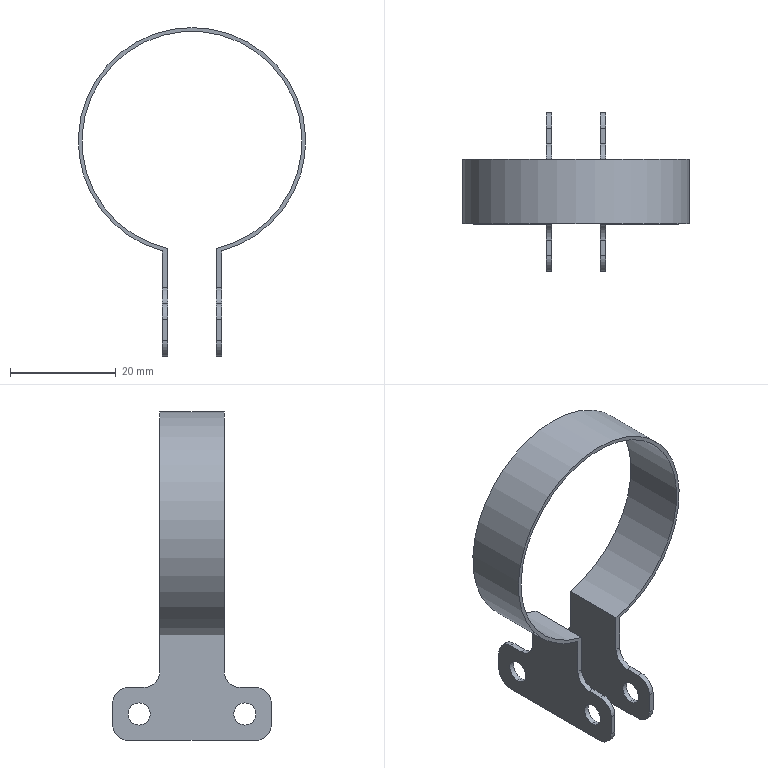Part | SolidWorks | features Extrusion 1, ICE 1, MirrorPattern 1 | 1 solid | 38 faces | box 43 x 30 x 62.202 mm | volume 1832 mm3 | cylinder 22 | plane 16 | commonest cylinder face diameters 6 x12 4.2 x8 41.6 x1 43 x1
STEP:
#1=CARTESIAN_POINT('',(5.6,16.1,-33.602));
#2=VERTEX_POINT('',#1);
#3=CARTESIAN_POINT('',(5.6,16.1,-37.802));
#4=VERTEX_POINT('',#3);
#5=CARTESIAN_POINT('',(5.6,16.1,-35.702));
#6=DIRECTION('',(1.,0.,0.));
#7=DIRECTION('',(0.,0.,-1.));
#8=AXIS2_PLACEMENT_3D('',#5,#6,#7);
#9=CIRCLE('',#8,2.1);
#10=EDGE_CURVE('',#2,#4,#9,.T.);
#11=ORIENTED_EDGE('',*,*,#10,.T.);
#12=CARTESIAN_POINT('',(4.6,16.1,-37.802));
#13=VERTEX_POINT('',#12);
#14=CARTESIAN_POINT('',(5.6,16.1,-37.802));
#15=DIRECTION('',(-1.,0.,0.));
#16=VECTOR('',#15,1000.);
#17=LINE('',#14,#16);
#18=EDGE_CURVE('',#4,#13,#17,.T.);
#19=ORIENTED_EDGE('',*,*,#18,.T.);
#20=CARTESIAN_POINT('',(4.6,16.1,-33.602));
#21=VERTEX_POINT('',#20);
#22=CARTESIAN_POINT('',(4.6,16.1,-35.702));
#23=DIRECTION('',(1.,0.,0.));
#24=DIRECTION('',(0.,0.,-1.));
#25=AXIS2_PLACEMENT_3D('',#22,#23,#24);
#26=CIRCLE('',#25,2.1);
#27=EDGE_CURVE('',#21,#13,#26,.T.);
#28=ORIENTED_EDGE('',*,*,#27,.F.);
#29=CARTESIAN_POINT('',(5.6,16.1,-33.602));
#30=DIRECTION('',(-1.,0.,0.));
#31=VECTOR('',#30,1000.);
#32=LINE('',#29,#31);
#33=EDGE_CURVE('',#2,#21,#32,.T.);
#34=ORIENTED_EDGE('',*,*,#33,.F.);
#35=EDGE_LOOP('',(#11,#19,#28,#34));
#36=FACE_OUTER_BOUND('',#35,.T.);
#37=CARTESIAN_POINT('',(5.6,16.1,-35.702));
#38=DIRECTION('',(-1.,0.,0.));
#39=DIRECTION('',(0.,0.,1.));
#40=AXIS2_PLACEMENT_3D('',#37,#38,#39);
#41=CYLINDRICAL_SURFACE('',#40,2.1);
#42=ADVANCED_FACE('',(#36),#41,.F.);
#43=CARTESIAN_POINT('',(5.6,-3.9,-33.602));
#44=VERTEX_POINT('',#43);
#45=CARTESIAN_POINT('',(5.6,-3.9,-37.802));
#46=VERTEX_POINT('',#45);
#47=CARTESIAN_POINT('',(5.6,-3.9,-35.702));
#48=DIRECTION('',(1.,0.,0.));
#49=DIRECTION('',(0.,0.,-1.));
#50=AXIS2_PLACEMENT_3D('',#47,#48,#49);
#51=CIRCLE('',#50,2.1);
#52=EDGE_CURVE('',#44,#46,#51,.T.);
#53=ORIENTED_EDGE('',*,*,#52,.T.);
#54=CARTESIAN_POINT('',(4.6,-3.9,-37.802));
#55=VERTEX_POINT('',#54);
#56=CARTESIAN_POINT('',(5.6,-3.9,-37.802));
#57=DIRECTION('',(-1.,0.,0.));
#58=VECTOR('',#57,1000.);
#59=LINE('',#56,#58);
#60=EDGE_CURVE('',#46,#55,#59,.T.);
#61=ORIENTED_EDGE('',*,*,#60,.T.);
#62=CARTESIAN_POINT('',(4.6,-3.9,-33.602));
#63=VERTEX_POINT('',#62);
#64=CARTESIAN_POINT('',(4.6,-3.9,-35.702));
#65=DIRECTION('',(1.,0.,0.));
#66=DIRECTION('',(0.,0.,-1.));
#67=AXIS2_PLACEMENT_3D('',#64,#65,#66);
#68=CIRCLE('',#67,2.1);
#69=EDGE_CURVE('',#63,#55,#68,.T.);
#70=ORIENTED_EDGE('',*,*,#69,.F.);
#71=CARTESIAN_POINT('',(5.6,-3.9,-33.602));
#72=DIRECTION('',(-1.,0.,0.));
#73=VECTOR('',#72,1000.);
#74=LINE('',#71,#73);
#75=EDGE_CURVE('',#44,#63,#74,.T.);
#76=ORIENTED_EDGE('',*,*,#75,.F.);
#77=EDGE_LOOP('',(#53,#61,#70,#76));
#78=FACE_OUTER_BOUND('',#77,.T.);
#79=CARTESIAN_POINT('',(5.6,-3.9,-35.702));
#80=DIRECTION('',(-1.,0.,0.));
#81=DIRECTION('',(0.,0.,1.));
#82=AXIS2_PLACEMENT_3D('',#79,#80,#81);
#83=CYLINDRICAL_SURFACE('',#82,2.1);
#84=ADVANCED_FACE('',(#78),#83,.F.);
#85=CARTESIAN_POINT('',(-5.6,16.1,-33.602));
#86=VERTEX_POINT('',#85);
#87=CARTESIAN_POINT('',(-5.6,16.1,-37.802));
#88=VERTEX_POINT('',#87);
#89=CARTESIAN_POINT('',(-5.6,16.1,-35.702));
#90=DIRECTION('',(1.,0.,0.));
#91=DIRECTION('',(0.,0.,-1.));
#92=AXIS2_PLACEMENT_3D('',#89,#90,#91);
#93=CIRCLE('',#92,2.1);
#94=EDGE_CURVE('',#86,#88,#93,.T.);
#95=ORIENTED_EDGE('',*,*,#94,.F.);
#96=CARTESIAN_POINT('',(-4.6,16.1,-33.602));
#97=VERTEX_POINT('',#96);
#98=CARTESIAN_POINT('',(-5.6,16.1,-33.602));
#99=DIRECTION('',(1.,0.,0.));
#100=VECTOR('',#99,1000.);
#101=LINE('',#98,#100);
#102=EDGE_CURVE('',#86,#97,#101,.T.);
#103=ORIENTED_EDGE('',*,*,#102,.T.);
#104=CARTESIAN_POINT('',(-4.6,16.1,-37.802));
#105=VERTEX_POINT('',#104);
#106=CARTESIAN_POINT('',(-4.6,16.1,-35.702));
#107=DIRECTION('',(1.,0.,0.));
#108=DIRECTION('',(0.,0.,-1.));
#109=AXIS2_PLACEMENT_3D('',#106,#107,#108);
#110=CIRCLE('',#109,2.1);
#111=EDGE_CURVE('',#97,#105,#110,.T.);
#112=ORIENTED_EDGE('',*,*,#111,.T.);
#113=CARTESIAN_POINT('',(-5.6,16.1,-37.802));
#114=DIRECTION('',(1.,0.,0.));
#115=VECTOR('',#114,1000.);
#116=LINE('',#113,#115);
#117=EDGE_CURVE('',#88,#105,#116,.T.);
#118=ORIENTED_EDGE('',*,*,#117,.F.);
#119=EDGE_LOOP('',(#95,#103,#112,#118));
#120=FACE_OUTER_BOUND('',#119,.T.);
#121=CARTESIAN_POINT('',(-5.6,16.1,-35.702));
#122=DIRECTION('',(1.,0.,0.));
#123=DIRECTION('',(0.,0.,-1.));
#124=AXIS2_PLACEMENT_3D('',#121,#122,#123);
#125=CYLINDRICAL_SURFACE('',#124,2.1);
#126=ADVANCED_FACE('',(#120),#125,.F.);
#127=CARTESIAN_POINT('',(-5.6,-3.9,-33.602));
#128=VERTEX_POINT('',#127);
#129=CARTESIAN_POINT('',(-5.6,-3.9,-37.802));
#130=VERTEX_POINT('',#129);
#131=CARTESIAN_POINT('',(-5.6,-3.9,-35.702));
#132=DIRECTION('',(1.,0.,0.));
#133=DIRECTION('',(0.,0.,-1.));
#134=AXIS2_PLACEMENT_3D('',#131,#132,#133);
#135=CIRCLE('',#134,2.1);
#136=EDGE_CURVE('',#128,#130,#135,.T.);
#137=ORIENTED_EDGE('',*,*,#136,.F.);
#138=CARTESIAN_POINT('',(-4.6,-3.9,-33.602));
#139=VERTEX_POINT('',#138);
#140=CARTESIAN_POINT('',(-5.6,-3.9,-33.602));
#141=DIRECTION('',(1.,0.,0.));
#142=VECTOR('',#141,1000.);
#143=LINE('',#140,#142);
#144=EDGE_CURVE('',#128,#139,#143,.T.);
#145=ORIENTED_EDGE('',*,*,#144,.T.);
#146=CARTESIAN_POINT('',(-4.6,-3.9,-37.802));
#147=VERTEX_POINT('',#146);
#148=CARTESIAN_POINT('',(-4.6,-3.9,-35.702));
#149=DIRECTION('',(1.,0.,0.));
#150=DIRECTION('',(0.,0.,-1.));
#151=AXIS2_PLACEMENT_3D('',#148,#149,#150);
#152=CIRCLE('',#151,2.1);
#153=EDGE_CURVE('',#139,#147,#152,.T.);
#154=ORIENTED_EDGE('',*,*,#153,.T.);
#155=CARTESIAN_POINT('',(-5.6,-3.9,-37.802));
#156=DIRECTION('',(1.,0.,0.));
#157=VECTOR('',#156,1000.);
#158=LINE('',#155,#157);
#159=EDGE_CURVE('',#130,#147,#158,.T.);
#160=ORIENTED_EDGE('',*,*,#159,.F.);
#161=EDGE_LOOP('',(#137,#145,#154,#160));
#162=FACE_OUTER_BOUND('',#161,.T.);
#163=CARTESIAN_POINT('',(-5.6,-3.9,-35.702));
#164=DIRECTION('',(1.,0.,0.));
#165=DIRECTION('',(0.,0.,-1.));
#166=AXIS2_PLACEMENT_3D('',#163,#164,#165);
#167=CYLINDRICAL_SURFACE('',#166,2.1);
#168=ADVANCED_FACE('',(#162),#167,.F.);
#169=CARTESIAN_POINT('',(5.6,12.2,-20.758));
#170=VERTEX_POINT('',#169);
#171=CARTESIAN_POINT('',(5.6,0.,-20.758));
#172=VERTEX_POINT('',#171);
#173=CARTESIAN_POINT('',(5.6,12.2,-20.758));
#174=DIRECTION('',(0.,-1.,0.));
#175=VECTOR('',#174,1000.);
#176=LINE('',#173,#175);
#177=EDGE_CURVE('',#170,#172,#176,.T.);
#178=ORIENTED_EDGE('',*,*,#177,.F.);
#179=CARTESIAN_POINT('',(-5.6,12.2,-20.758));
#180=VERTEX_POINT('',#179);
#181=CARTESIAN_POINT('',(0.,12.2,0.));
#182=DIRECTION('',(0.,1.,0.));
#183=DIRECTION('',(0.,0.,1.));
#184=AXIS2_PLACEMENT_3D('',#181,#182,#183);
#185=CIRCLE('',#184,21.5);
#186=EDGE_CURVE('',#180,#170,#185,.T.);
#187=ORIENTED_EDGE('',*,*,#186,.F.);
#188=CARTESIAN_POINT('',(-5.6,0.,-20.758));
#189=VERTEX_POINT('',#188);
#190=CARTESIAN_POINT('',(-5.6,12.2,-20.758));
#191=DIRECTION('',(0.,1.,0.));
#192=VECTOR('',#191,1000.);
#193=LINE('',#190,#192);
#194=EDGE_CURVE('',#189,#180,#193,.T.);
#195=ORIENTED_EDGE('',*,*,#194,.F.);
#196=CARTESIAN_POINT('',(0.,0.,0.));
#197=DIRECTION('',(0.,1.,0.));
#198=DIRECTION('',(0.,0.,1.));
#199=AXIS2_PLACEMENT_3D('',#196,#197,#198);
#200=CIRCLE('',#199,21.5);
#201=EDGE_CURVE('',#189,#172,#200,.T.);
#202=ORIENTED_EDGE('',*,*,#201,.T.);
#203=EDGE_LOOP('',(#178,#187,#195,#202));
#204=FACE_OUTER_BOUND('',#203,.T.);
#205=CARTESIAN_POINT('',(0.,12.2,0.));
#206=DIRECTION('',(0.,-1.,0.));
#207=DIRECTION('',(0.,0.,-1.));
#208=AXIS2_PLACEMENT_3D('',#205,#206,#207);
#209=CYLINDRICAL_SURFACE('',#208,21.5);
#210=ADVANCED_FACE('',(#204),#209,.T.);
#211=CARTESIAN_POINT('',(4.6,0.,-27.702));
#212=VERTEX_POINT('',#211);
#213=CARTESIAN_POINT('',(4.6,0.,-20.285));
#214=VERTEX_POINT('',#213);
#215=CARTESIAN_POINT('',(4.6,0.,-20.285));
#216=DIRECTION('',(0.,0.,1.));
#217=VECTOR('',#216,1000.);
#218=LINE('',#215,#217);
#219=EDGE_CURVE('',#212,#214,#218,.T.);
#220=ORIENTED_EDGE('',*,*,#219,.T.);
#221=CARTESIAN_POINT('',(4.6,12.2,-20.285));
#222=VERTEX_POINT('',#221);
#223=CARTESIAN_POINT('',(4.6,12.2,-20.285));
#224=DIRECTION('',(0.,-1.,0.));
#225=VECTOR('',#224,1000.);
#226=LINE('',#223,#225);
#227=EDGE_CURVE('',#222,#214,#226,.T.);
#228=ORIENTED_EDGE('',*,*,#227,.F.);
#229=CARTESIAN_POINT('',(4.6,12.2,-27.702));
#230=VERTEX_POINT('',#229);
#231=CARTESIAN_POINT('',(4.6,12.2,-20.285));
#232=DIRECTION('',(0.,0.,1.));
#233=VECTOR('',#232,1000.);
#234=LINE('',#231,#233);
#235=EDGE_CURVE('',#230,#222,#234,.T.);
#236=ORIENTED_EDGE('',*,*,#235,.F.);
#237=CARTESIAN_POINT('',(4.6,15.2,-30.702));
#238=VERTEX_POINT('',#237);
#239=CARTESIAN_POINT('',(4.6,15.2,-27.702));
#240=DIRECTION('',(-1.,0.,0.));
#241=DIRECTION('',(0.,0.,-1.));
#242=AXIS2_PLACEMENT_3D('',#239,#240,#241);
#243=CIRCLE('',#242,3.);
#244=EDGE_CURVE('',#238,#230,#243,.T.);
#245=ORIENTED_EDGE('',*,*,#244,.F.);
#246=CARTESIAN_POINT('',(4.6,18.1,-30.702));
#247=VERTEX_POINT('',#246);
#248=CARTESIAN_POINT('',(4.6,0.,-30.702));
#249=DIRECTION('',(0.,-1.,0.));
#250=VECTOR('',#249,1000.);
#251=LINE('',#248,#250);
#252=EDGE_CURVE('',#247,#238,#251,.T.);
#253=ORIENTED_EDGE('',*,*,#252,.F.);
#254=CARTESIAN_POINT('',(4.6,21.1,-33.702));
#255=VERTEX_POINT('',#254);
#256=CARTESIAN_POINT('',(4.6,18.1,-33.702));
#257=DIRECTION('',(1.,0.,0.));
#258=DIRECTION('',(0.,0.,-1.));
#259=AXIS2_PLACEMENT_3D('',#256,#257,#258);
#260=CIRCLE('',#259,3.);
#261=EDGE_CURVE('',#255,#247,#260,.T.);
#262=ORIENTED_EDGE('',*,*,#261,.F.);
#263=CARTESIAN_POINT('',(4.6,21.1,-37.702));
#264=VERTEX_POINT('',#263);
#265=CARTESIAN_POINT('',(4.6,21.1,0.));
#266=DIRECTION('',(0.,0.,1.));
#267=VECTOR('',#266,1000.);
#268=LINE('',#265,#267);
#269=EDGE_CURVE('',#264,#255,#268,.T.);
#270=ORIENTED_EDGE('',*,*,#269,.F.);
#271=CARTESIAN_POINT('',(4.6,18.1,-40.702));
#272=VERTEX_POINT('',#271);
#273=CARTESIAN_POINT('',(4.6,18.1,-37.702));
#274=DIRECTION('',(1.,0.,0.));
#275=DIRECTION('',(0.,0.,-1.));
#276=AXIS2_PLACEMENT_3D('',#273,#274,#275);
#277=CIRCLE('',#276,3.);
#278=EDGE_CURVE('',#272,#264,#277,.T.);
#279=ORIENTED_EDGE('',*,*,#278,.F.);
#280=CARTESIAN_POINT('',(4.6,-5.9,-40.702));
#281=VERTEX_POINT('',#280);
#282=CARTESIAN_POINT('',(4.6,0.,-40.702));
#283=DIRECTION('',(0.,1.,0.));
#284=VECTOR('',#283,1000.);
#285=LINE('',#282,#284);
#286=EDGE_CURVE('',#281,#272,#285,.T.);
#287=ORIENTED_EDGE('',*,*,#286,.F.);
#288=CARTESIAN_POINT('',(4.6,-8.9,-37.702));
#289=VERTEX_POINT('',#288);
#290=CARTESIAN_POINT('',(4.6,-5.9,-37.702));
#291=DIRECTION('',(1.,0.,0.));
#292=DIRECTION('',(0.,0.,-1.));
#293=AXIS2_PLACEMENT_3D('',#290,#291,#292);
#294=CIRCLE('',#293,3.);
#295=EDGE_CURVE('',#289,#281,#294,.T.);
#296=ORIENTED_EDGE('',*,*,#295,.F.);
#297=CARTESIAN_POINT('',(4.6,-8.9,-33.702));
#298=VERTEX_POINT('',#297);
#299=CARTESIAN_POINT('',(4.6,-8.9,0.));
#300=DIRECTION('',(0.,0.,-1.));
#301=VECTOR('',#300,1000.);
#302=LINE('',#299,#301);
#303=EDGE_CURVE('',#298,#289,#302,.T.);
#304=ORIENTED_EDGE('',*,*,#303,.F.);
#305=CARTESIAN_POINT('',(4.6,-5.9,-30.702));
#306=VERTEX_POINT('',#305);
#307=CARTESIAN_POINT('',(4.6,-5.9,-33.702));
#308=DIRECTION('',(1.,0.,0.));
#309=DIRECTION('',(0.,0.,-1.));
#310=AXIS2_PLACEMENT_3D('',#307,#308,#309);
#311=CIRCLE('',#310,3.);
#312=EDGE_CURVE('',#306,#298,#311,.T.);
#313=ORIENTED_EDGE('',*,*,#312,.F.);
#314=CARTESIAN_POINT('',(4.6,-3.,-30.702));
#315=VERTEX_POINT('',#314);
#316=CARTESIAN_POINT('',(4.6,0.,-30.702));
#317=DIRECTION('',(0.,-1.,0.));
#318=VECTOR('',#317,1000.);
#319=LINE('',#316,#318);
#320=EDGE_CURVE('',#315,#306,#319,.T.);
#321=ORIENTED_EDGE('',*,*,#320,.F.);
#322=CARTESIAN_POINT('',(4.6,-3.,-27.702));
#323=DIRECTION('',(-1.,0.,0.));
#324=DIRECTION('',(0.,0.,-1.));
#325=AXIS2_PLACEMENT_3D('',#322,#323,#324);
#326=CIRCLE('',#325,3.);
#327=EDGE_CURVE('',#212,#315,#326,.T.);
#328=ORIENTED_EDGE('',*,*,#327,.F.);
#329=EDGE_LOOP('',(#220,#228,#236,#245,#253,#262,#270,#279,#287,#296,#304,#313,#321,#328));
#330=FACE_OUTER_BOUND('',#329,.T.);
#331=ORIENTED_EDGE('',*,*,#69,.T.);
#332=CARTESIAN_POINT('',(4.6,-3.9,-35.702));
#333=DIRECTION('',(1.,0.,0.));
#334=DIRECTION('',(0.,0.,-1.));
#335=AXIS2_PLACEMENT_3D('',#332,#333,#334);
#336=CIRCLE('',#335,2.1);
#337=EDGE_CURVE('',#55,#63,#336,.T.);
#338=ORIENTED_EDGE('',*,*,#337,.T.);
#339=EDGE_LOOP('',(#331,#338));
#340=FACE_BOUND('',#339,.T.);
#341=ORIENTED_EDGE('',*,*,#27,.T.);
#342=CARTESIAN_POINT('',(4.6,16.1,-35.702));
#343=DIRECTION('',(1.,0.,0.));
#344=DIRECTION('',(0.,0.,-1.));
#345=AXIS2_PLACEMENT_3D('',#342,#343,#344);
#346=CIRCLE('',#345,2.1);
#347=EDGE_CURVE('',#13,#21,#346,.T.);
#348=ORIENTED_EDGE('',*,*,#347,.T.);
#349=EDGE_LOOP('',(#341,#348));
#350=FACE_BOUND('',#349,.T.);
#351=CARTESIAN_POINT('',(4.6,12.2,-20.285));
#352=DIRECTION('',(1.,0.,0.));
#353=DIRECTION('',(0.,0.,-1.));
#354=AXIS2_PLACEMENT_3D('',#351,#352,#353);
#355=PLANE('',#354);
#356=ADVANCED_FACE('',(#330,#340,#350),#355,.F.);
#357=CARTESIAN_POINT('',(-4.6,0.,-20.285));
#358=VERTEX_POINT('',#357);
#359=CARTESIAN_POINT('',(0.,0.,0.));
#360=DIRECTION('',(0.,-1.,0.));
#361=DIRECTION('',(0.,0.,1.));
#362=AXIS2_PLACEMENT_3D('',#359,#360,#361);
#363=CIRCLE('',#362,20.8);
#364=EDGE_CURVE('',#214,#358,#363,.T.);
#365=ORIENTED_EDGE('',*,*,#364,.T.);
#366=CARTESIAN_POINT('',(-4.6,12.2,-20.285));
#367=VERTEX_POINT('',#366);
#368=CARTESIAN_POINT('',(-4.6,12.2,-20.285));
#369=DIRECTION('',(0.,-1.,0.));
#370=VECTOR('',#369,1000.);
#371=LINE('',#368,#370);
#372=EDGE_CURVE('',#367,#358,#371,.T.);
#373=ORIENTED_EDGE('',*,*,#372,.F.);
#374=CARTESIAN_POINT('',(0.,12.2,0.));
#375=DIRECTION('',(0.,-1.,0.));
#376=DIRECTION('',(0.,0.,1.));
#377=AXIS2_PLACEMENT_3D('',#374,#375,#376);
#378=CIRCLE('',#377,20.8);
#379=EDGE_CURVE('',#222,#367,#378,.T.);
#380=ORIENTED_EDGE('',*,*,#379,.F.);
#381=ORIENTED_EDGE('',*,*,#227,.T.);
#382=EDGE_LOOP('',(#365,#373,#380,#381));
#383=FACE_OUTER_BOUND('',#382,.T.);
#384=CARTESIAN_POINT('',(0.,12.2,0.));
#385=DIRECTION('',(0.,-1.,0.));
#386=DIRECTION('',(0.,0.,-1.));
#387=AXIS2_PLACEMENT_3D('',#384,#385,#386);
#388=CYLINDRICAL_SURFACE('',#387,20.8);
#389=ADVANCED_FACE('',(#383),#388,.F.);
#390=CARTESIAN_POINT('',(-4.6,0.,-27.702));
#391=VERTEX_POINT('',#390);
#392=CARTESIAN_POINT('',(-4.6,0.,-20.285));
#393=DIRECTION('',(0.,0.,-1.));
#394=VECTOR('',#393,1000.);
#395=LINE('',#392,#394);
#396=EDGE_CURVE('',#358,#391,#395,.T.);
#397=ORIENTED_EDGE('',*,*,#396,.T.);
#398=CARTESIAN_POINT('',(-4.6,-3.,-30.702));
#399=VERTEX_POINT('',#398);
#400=CARTESIAN_POINT('',(-4.6,-3.,-27.702));
#401=DIRECTION('',(-1.,0.,0.));
#402=DIRECTION('',(0.,0.,-1.));
#403=AXIS2_PLACEMENT_3D('',#400,#401,#402);
#404=CIRCLE('',#403,3.);
#405=EDGE_CURVE('',#391,#399,#404,.T.);
#406=ORIENTED_EDGE('',*,*,#405,.T.);
#407=CARTESIAN_POINT('',(-4.6,-5.9,-30.702));
#408=VERTEX_POINT('',#407);
#409=CARTESIAN_POINT('',(-4.6,0.,-30.702));
#410=DIRECTION('',(0.,-1.,0.));
#411=VECTOR('',#410,1000.);
#412=LINE('',#409,#411);
#413=EDGE_CURVE('',#399,#408,#412,.T.);
#414=ORIENTED_EDGE('',*,*,#413,.T.);
#415=CARTESIAN_POINT('',(-4.6,-8.9,-33.702));
#416=VERTEX_POINT('',#415);
#417=CARTESIAN_POINT('',(-4.6,-5.9,-33.702));
#418=DIRECTION('',(1.,0.,0.));
#419=DIRECTION('',(0.,0.,-1.));
#420=AXIS2_PLACEMENT_3D('',#417,#418,#419);
#421=CIRCLE('',#420,3.);
#422=EDGE_CURVE('',#408,#416,#421,.T.);
#423=ORIENTED_EDGE('',*,*,#422,.T.);
#424=CARTESIAN_POINT('',(-4.6,-8.9,-37.702));
#425=VERTEX_POINT('',#424);
#426=CARTESIAN_POINT('',(-4.6,-8.9,0.));
#427=DIRECTION('',(0.,0.,-1.));
#428=VECTOR('',#427,1000.);
#429=LINE('',#426,#428);
#430=EDGE_CURVE('',#416,#425,#429,.T.);
#431=ORIENTED_EDGE('',*,*,#430,.T.);
#432=CARTESIAN_POINT('',(-4.6,-5.9,-40.702));
#433=VERTEX_POINT('',#432);
#434=CARTESIAN_POINT('',(-4.6,-5.9,-37.702));
#435=DIRECTION('',(1.,0.,0.));
#436=DIRECTION('',(0.,0.,-1.));
#437=AXIS2_PLACEMENT_3D('',#434,#435,#436);
#438=CIRCLE('',#437,3.);
#439=EDGE_CURVE('',#425,#433,#438,.T.);
#440=ORIENTED_EDGE('',*,*,#439,.T.);
#441=CARTESIAN_POINT('',(-4.6,18.1,-40.702));
#442=VERTEX_POINT('',#441);
#443=CARTESIAN_POINT('',(-4.6,0.,-40.702));
#444=DIRECTION('',(0.,1.,0.));
#445=VECTOR('',#444,1000.);
#446=LINE('',#443,#445);
#447=EDGE_CURVE('',#433,#442,#446,.T.);
#448=ORIENTED_EDGE('',*,*,#447,.T.);
#449=CARTESIAN_POINT('',(-4.6,21.1,-37.702));
#450=VERTEX_POINT('',#449);
#451=CARTESIAN_POINT('',(-4.6,18.1,-37.702));
#452=DIRECTION('',(1.,0.,0.));
#453=DIRECTION('',(0.,0.,-1.));
#454=AXIS2_PLACEMENT_3D('',#451,#452,#453);
#455=CIRCLE('',#454,3.);
#456=EDGE_CURVE('',#442,#450,#455,.T.);
#457=ORIENTED_EDGE('',*,*,#456,.T.);
#458=CARTESIAN_POINT('',(-4.6,21.1,-33.702));
#459=VERTEX_POINT('',#458);
#460=CARTESIAN_POINT('',(-4.6,21.1,0.));
#461=DIRECTION('',(0.,0.,1.));
#462=VECTOR('',#461,1000.);
#463=LINE('',#460,#462);
#464=EDGE_CURVE('',#450,#459,#463,.T.);
#465=ORIENTED_EDGE('',*,*,#464,.T.);
#466=CARTESIAN_POINT('',(-4.6,18.1,-30.702));
#467=VERTEX_POINT('',#466);
#468=CARTESIAN_POINT('',(-4.6,18.1,-33.702));
#469=DIRECTION('',(1.,0.,0.));
#470=DIRECTION('',(0.,0.,-1.));
#471=AXIS2_PLACEMENT_3D('',#468,#469,#470);
#472=CIRCLE('',#471,3.);
#473=EDGE_CURVE('',#459,#467,#472,.T.);
#474=ORIENTED_EDGE('',*,*,#473,.T.);
#475=CARTESIAN_POINT('',(-4.6,15.2,-30.702));
#476=VERTEX_POINT('',#475);
#477=CARTESIAN_POINT('',(-4.6,0.,-30.702));
#478=DIRECTION('',(0.,-1.,0.));
#479=VECTOR('',#478,1000.);
#480=LINE('',#477,#479);
#481=EDGE_CURVE('',#467,#476,#480,.T.);
#482=ORIENTED_EDGE('',*,*,#481,.T.);
#483=CARTESIAN_POINT('',(-4.6,12.2,-27.702));
#484=VERTEX_POINT('',#483);
#485=CARTESIAN_POINT('',(-4.6,15.2,-27.702));
#486=DIRECTION('',(-1.,0.,0.));
#487=DIRECTION('',(0.,0.,-1.));
#488=AXIS2_PLACEMENT_3D('',#485,#486,#487);
#489=CIRCLE('',#488,3.);
#490=EDGE_CURVE('',#476,#484,#489,.T.);
#491=ORIENTED_EDGE('',*,*,#490,.T.);
#492=CARTESIAN_POINT('',(-4.6,12.2,-20.285));
#493=DIRECTION('',(0.,0.,-1.));
#494=VECTOR('',#493,1000.);
#495=LINE('',#492,#494);
#496=EDGE_CURVE('',#367,#484,#495,.T.);
#497=ORIENTED_EDGE('',*,*,#496,.F.);
#498=ORIENTED_EDGE('',*,*,#372,.T.);
#499=EDGE_LOOP('',(#397,#406,#414,#423,#431,#440,#448,#457,#465,#474,#482,#491,#497,#498));
#500=FACE_OUTER_BOUND('',#499,.T.);
#501=CARTESIAN_POINT('',(-4.6,-3.9,-35.702));
#502=DIRECTION('',(1.,0.,0.));
#503=DIRECTION('',(0.,0.,-1.));
#504=AXIS2_PLACEMENT_3D('',#501,#502,#503);
#505=CIRCLE('',#504,2.1);
#506=EDGE_CURVE('',#147,#139,#505,.T.);
#507=ORIENTED_EDGE('',*,*,#506,.F.);
#508=ORIENTED_EDGE('',*,*,#153,.F.);
#509=EDGE_LOOP('',(#507,#508));
#510=FACE_BOUND('',#509,.T.);
#511=CARTESIAN_POINT('',(-4.6,16.1,-35.702));
#512=DIRECTION('',(1.,0.,0.));
#513=DIRECTION('',(0.,0.,-1.));
#514=AXIS2_PLACEMENT_3D('',#511,#512,#513);
#515=CIRCLE('',#514,2.1);
#516=EDGE_CURVE('',#105,#97,#515,.T.);
#517=ORIENTED_EDGE('',*,*,#516,.F.);
#518=ORIENTED_EDGE('',*,*,#111,.F.);
#519=EDGE_LOOP('',(#517,#518));
#520=FACE_BOUND('',#519,.T.);
#521=CARTESIAN_POINT('',(-4.6,12.2,-20.285));
#522=DIRECTION('',(-1.,0.,0.));
#523=DIRECTION('',(0.,0.,1.));
#524=AXIS2_PLACEMENT_3D('',#521,#522,#523);
#525=PLANE('',#524);
#526=ADVANCED_FACE('',(#500,#510,#520),#525,.F.);
#527=ORIENTED_EDGE('',*,*,#235,.T.);
#528=ORIENTED_EDGE('',*,*,#379,.T.);
#529=ORIENTED_EDGE('',*,*,#496,.T.);
#530=CARTESIAN_POINT('',(-5.6,12.2,-27.702));
#531=VERTEX_POINT('',#530);
#532=CARTESIAN_POINT('',(-5.6,12.2,-27.702));
#533=DIRECTION('',(1.,0.,0.));
#534=VECTOR('',#533,1000.);
#535=LINE('',#532,#534);
#536=EDGE_CURVE('',#531,#484,#535,.T.);
#537=ORIENTED_EDGE('',*,*,#536,.F.);
#538=CARTESIAN_POINT('',(-5.6,12.2,0.));
#539=DIRECTION('',(0.,0.,1.));
#540=VECTOR('',#539,1000.);
#541=LINE('',#538,#540);
#542=EDGE_CURVE('',#531,#180,#541,.T.);
#543=ORIENTED_EDGE('',*,*,#542,.T.);
#544=ORIENTED_EDGE('',*,*,#186,.T.);
#545=CARTESIAN_POINT('',(5.6,12.2,-27.702));
#546=VERTEX_POINT('',#545);
#547=CARTESIAN_POINT('',(5.6,12.2,0.));
#548=DIRECTION('',(0.,0.,1.));
#549=VECTOR('',#548,1000.);
#550=LINE('',#547,#549);
#551=EDGE_CURVE('',#546,#170,#550,.T.);
#552=ORIENTED_EDGE('',*,*,#551,.F.);
#553=CARTESIAN_POINT('',(5.6,12.2,-27.702));
#554=DIRECTION('',(-1.,0.,0.));
#555=VECTOR('',#554,1000.);
#556=LINE('',#553,#555);
#557=EDGE_CURVE('',#546,#230,#556,.T.);
#558=ORIENTED_EDGE('',*,*,#557,.T.);
#559=EDGE_LOOP('',(#527,#528,#529,#537,#543,#544,#552,#558));
#560=FACE_OUTER_BOUND('',#559,.T.);
#561=CARTESIAN_POINT('',(0.,12.2,0.));
#562=DIRECTION('',(0.,1.,0.));
#563=DIRECTION('',(0.,0.,1.));
#564=AXIS2_PLACEMENT_3D('',#561,#562,#563);
#565=PLANE('',#564);
#566=ADVANCED_FACE('',(#560),#565,.T.);
#567=ORIENTED_EDGE('',*,*,#364,.F.);
#568=ORIENTED_EDGE('',*,*,#219,.F.);
#569=CARTESIAN_POINT('',(5.6,0.,-27.702));
#570=VERTEX_POINT('',#569);
#571=CARTESIAN_POINT('',(5.6,0.,-27.702));
#572=DIRECTION('',(-1.,0.,0.));
#573=VECTOR('',#572,1000.);
#574=LINE('',#571,#573);
#575=EDGE_CURVE('',#570,#212,#574,.T.);
#576=ORIENTED_EDGE('',*,*,#575,.F.);
#577=CARTESIAN_POINT('',(5.6,0.,0.));
#578=DIRECTION('',(0.,0.,-1.));
#579=VECTOR('',#578,1000.);
#580=LINE('',#577,#579);
#581=EDGE_CURVE('',#172,#570,#580,.T.);
#582=ORIENTED_EDGE('',*,*,#581,.F.);
#583=ORIENTED_EDGE('',*,*,#201,.F.);
#584=CARTESIAN_POINT('',(-5.6,0.,-27.702));
#585=VERTEX_POINT('',#584);
#586=CARTESIAN_POINT('',(-5.6,0.,0.));
#587=DIRECTION('',(0.,0.,-1.));
#588=VECTOR('',#587,1000.);
#589=LINE('',#586,#588);
#590=EDGE_CURVE('',#189,#585,#589,.T.);
#591=ORIENTED_EDGE('',*,*,#590,.T.);
#592=CARTESIAN_POINT('',(-5.6,0.,-27.702));
#593=DIRECTION('',(1.,0.,0.));
#594=VECTOR('',#593,1000.);
#595=LINE('',#592,#594);
#596=EDGE_CURVE('',#585,#391,#595,.T.);
#597=ORIENTED_EDGE('',*,*,#596,.T.);
#598=ORIENTED_EDGE('',*,*,#396,.F.);
#599=EDGE_LOOP('',(#567,#568,#576,#582,#583,#591,#597,#598));
#600=FACE_OUTER_BOUND('',#599,.T.);
#601=CARTESIAN_POINT('',(0.,0.,0.));
#602=DIRECTION('',(0.,1.,0.));
#603=DIRECTION('',(0.,0.,1.));
#604=AXIS2_PLACEMENT_3D('',#601,#602,#603);
#605=PLANE('',#604);
#606=ADVANCED_FACE('',(#600),#605,.F.);
#607=CARTESIAN_POINT('',(-5.6,16.1,-35.702));
#608=DIRECTION('',(1.,0.,0.));
#609=DIRECTION('',(0.,0.,-1.));
#610=AXIS2_PLACEMENT_3D('',#607,#608,#609);
#611=CIRCLE('',#610,2.1);
#612=EDGE_CURVE('',#88,#86,#611,.T.);
#613=ORIENTED_EDGE('',*,*,#612,.T.);
#614=ORIENTED_EDGE('',*,*,#94,.T.);
#615=EDGE_LOOP('',(#613,#614));
#616=FACE_BOUND('',#615,.T.);
#617=CARTESIAN_POINT('',(-5.6,-3.9,-35.702));
#618=DIRECTION('',(1.,0.,0.));
#619=DIRECTION('',(0.,0.,-1.));
#620=AXIS2_PLACEMENT_3D('',#617,#618,#619);
#621=CIRCLE('',#620,2.1);
#622=EDGE_CURVE('',#130,#128,#621,.T.);
#623=ORIENTED_EDGE('',*,*,#622,.T.);
#624=ORIENTED_EDGE('',*,*,#136,.T.);
#625=EDGE_LOOP('',(#623,#624));
#626=FACE_BOUND('',#625,.T.);
#627=ORIENTED_EDGE('',*,*,#590,.F.);
#628=ORIENTED_EDGE('',*,*,#194,.T.);
#629=ORIENTED_EDGE('',*,*,#542,.F.);
#630=CARTESIAN_POINT('',(-5.6,15.2,-30.702));
#631=VERTEX_POINT('',#630);
#632=CARTESIAN_POINT('',(-5.6,15.2,-27.702));
#633=DIRECTION('',(-1.,0.,0.));
#634=DIRECTION('',(0.,0.,-1.));
#635=AXIS2_PLACEMENT_3D('',#632,#633,#634);
#636=CIRCLE('',#635,3.);
#637=EDGE_CURVE('',#631,#531,#636,.T.);
#638=ORIENTED_EDGE('',*,*,#637,.F.);
#639=CARTESIAN_POINT('',(-5.6,18.1,-30.702));
#640=VERTEX_POINT('',#639);
#641=CARTESIAN_POINT('',(-5.6,0.,-30.702));
#642=DIRECTION('',(0.,-1.,0.));
#643=VECTOR('',#642,1000.);
#644=LINE('',#641,#643);
#645=EDGE_CURVE('',#640,#631,#644,.T.);
#646=ORIENTED_EDGE('',*,*,#645,.F.);
#647=CARTESIAN_POINT('',(-5.6,21.1,-33.702));
#648=VERTEX_POINT('',#647);
#649=CARTESIAN_POINT('',(-5.6,18.1,-33.702));
#650=DIRECTION('',(1.,0.,0.));
#651=DIRECTION('',(0.,0.,-1.));
#652=AXIS2_PLACEMENT_3D('',#649,#650,#651);
#653=CIRCLE('',#652,3.);
#654=EDGE_CURVE('',#648,#640,#653,.T.);
#655=ORIENTED_EDGE('',*,*,#654,.F.);
#656=CARTESIAN_POINT('',(-5.6,21.1,-37.702));
#657=VERTEX_POINT('',#656);
#658=CARTESIAN_POINT('',(-5.6,21.1,0.));
#659=DIRECTION('',(0.,0.,1.));
#660=VECTOR('',#659,1000.);
#661=LINE('',#658,#660);
#662=EDGE_CURVE('',#657,#648,#661,.T.);
#663=ORIENTED_EDGE('',*,*,#662,.F.);
#664=CARTESIAN_POINT('',(-5.6,18.1,-40.702));
#665=VERTEX_POINT('',#664);
#666=CARTESIAN_POINT('',(-5.6,18.1,-37.702));
#667=DIRECTION('',(1.,0.,0.));
#668=DIRECTION('',(0.,0.,-1.));
#669=AXIS2_PLACEMENT_3D('',#666,#667,#668);
#670=CIRCLE('',#669,3.);
#671=EDGE_CURVE('',#665,#657,#670,.T.);
#672=ORIENTED_EDGE('',*,*,#671,.F.);
#673=CARTESIAN_POINT('',(-5.6,-5.9,-40.702));
#674=VERTEX_POINT('',#673);
#675=CARTESIAN_POINT('',(-5.6,0.,-40.702));
#676=DIRECTION('',(0.,1.,0.));
#677=VECTOR('',#676,1000.);
#678=LINE('',#675,#677);
#679=EDGE_CURVE('',#674,#665,#678,.T.);
#680=ORIENTED_EDGE('',*,*,#679,.F.);
#681=CARTESIAN_POINT('',(-5.6,-8.9,-37.702));
#682=VERTEX_POINT('',#681);
#683=CARTESIAN_POINT('',(-5.6,-5.9,-37.702));
#684=DIRECTION('',(1.,0.,0.));
#685=DIRECTION('',(0.,0.,-1.));
#686=AXIS2_PLACEMENT_3D('',#683,#684,#685);
#687=CIRCLE('',#686,3.);
#688=EDGE_CURVE('',#682,#674,#687,.T.);
#689=ORIENTED_EDGE('',*,*,#688,.F.);
#690=CARTESIAN_POINT('',(-5.6,-8.9,-33.702));
#691=VERTEX_POINT('',#690);
#692=CARTESIAN_POINT('',(-5.6,-8.9,0.));
#693=DIRECTION('',(0.,0.,-1.));
#694=VECTOR('',#693,1000.);
#695=LINE('',#692,#694);
#696=EDGE_CURVE('',#691,#682,#695,.T.);
#697=ORIENTED_EDGE('',*,*,#696,.F.);
#698=CARTESIAN_POINT('',(-5.6,-5.9,-30.702));
#699=VERTEX_POINT('',#698);
#700=CARTESIAN_POINT('',(-5.6,-5.9,-33.702));
#701=DIRECTION('',(1.,0.,0.));
#702=DIRECTION('',(0.,0.,-1.));
#703=AXIS2_PLACEMENT_3D('',#700,#701,#702);
#704=CIRCLE('',#703,3.);
#705=EDGE_CURVE('',#699,#691,#704,.T.);
#706=ORIENTED_EDGE('',*,*,#705,.F.);
#707=CARTESIAN_POINT('',(-5.6,-3.,-30.702));
#708=VERTEX_POINT('',#707);
#709=CARTESIAN_POINT('',(-5.6,0.,-30.702));
#710=DIRECTION('',(0.,-1.,0.));
#711=VECTOR('',#710,1000.);
#712=LINE('',#709,#711);
#713=EDGE_CURVE('',#708,#699,#712,.T.);
#714=ORIENTED_EDGE('',*,*,#713,.F.);
#715=CARTESIAN_POINT('',(-5.6,-3.,-27.702));
#716=DIRECTION('',(-1.,0.,0.));
#717=DIRECTION('',(0.,0.,-1.));
#718=AXIS2_PLACEMENT_3D('',#715,#716,#717);
#719=CIRCLE('',#718,3.);
#720=EDGE_CURVE('',#585,#708,#719,.T.);
#721=ORIENTED_EDGE('',*,*,#720,.F.);
#722=EDGE_LOOP('',(#627,#628,#629,#638,#646,#655,#663,#672,#680,#689,#697,#706,#714,#721));
#723=FACE_OUTER_BOUND('',#722,.T.);
#724=CARTESIAN_POINT('',(-5.6,0.,0.));
#725=DIRECTION('',(1.,0.,0.));
#726=DIRECTION('',(0.,0.,-1.));
#727=AXIS2_PLACEMENT_3D('',#724,#725,#726);
#728=PLANE('',#727);
#729=ADVANCED_FACE('',(#616,#626,#723),#728,.F.);
#730=ORIENTED_EDGE('',*,*,#481,.F.);
#731=CARTESIAN_POINT('',(-5.6,18.1,-30.702));
#732=DIRECTION('',(1.,0.,0.));
#733=VECTOR('',#732,1000.);
#734=LINE('',#731,#733);
#735=EDGE_CURVE('',#640,#467,#734,.T.);
#736=ORIENTED_EDGE('',*,*,#735,.F.);
#737=ORIENTED_EDGE('',*,*,#645,.T.);
#738=CARTESIAN_POINT('',(-5.6,15.2,-30.702));
#739=DIRECTION('',(1.,0.,0.));
#740=VECTOR('',#739,1000.);
#741=LINE('',#738,#740);
#742=EDGE_CURVE('',#631,#476,#741,.T.);
#743=ORIENTED_EDGE('',*,*,#742,.T.);
#744=EDGE_LOOP('',(#730,#736,#737,#743));
#745=FACE_OUTER_BOUND('',#744,.T.);
#746=CARTESIAN_POINT('',(-5.6,0.,-30.702));
#747=DIRECTION('',(0.,0.,1.));
#748=DIRECTION('',(1.,0.,0.));
#749=AXIS2_PLACEMENT_3D('',#746,#747,#748);
#750=PLANE('',#749);
#751=ADVANCED_FACE('',(#745),#750,.T.);
#752=ORIENTED_EDGE('',*,*,#473,.F.);
#753=CARTESIAN_POINT('',(-5.6,21.1,-33.702));
#754=DIRECTION('',(1.,0.,0.));
#755=VECTOR('',#754,1000.);
#756=LINE('',#753,#755);
#757=EDGE_CURVE('',#648,#459,#756,.T.);
#758=ORIENTED_EDGE('',*,*,#757,.F.);
#759=ORIENTED_EDGE('',*,*,#654,.T.);
#760=ORIENTED_EDGE('',*,*,#735,.T.);
#761=EDGE_LOOP('',(#752,#758,#759,#760));
#762=FACE_OUTER_BOUND('',#761,.T.);
#763=CARTESIAN_POINT('',(-5.6,18.1,-33.702));
#764=DIRECTION('',(1.,0.,0.));
#765=DIRECTION('',(0.,0.,-1.));
#766=AXIS2_PLACEMENT_3D('',#763,#764,#765);
#767=CYLINDRICAL_SURFACE('',#766,3.);
#768=ADVANCED_FACE('',(#762),#767,.T.);
#769=ORIENTED_EDGE('',*,*,#464,.F.);
#770=CARTESIAN_POINT('',(-5.6,21.1,-37.702));
#771=DIRECTION('',(1.,0.,0.));
#772=VECTOR('',#771,1000.);
#773=LINE('',#770,#772);
#774=EDGE_CURVE('',#657,#450,#773,.T.);
#775=ORIENTED_EDGE('',*,*,#774,.F.);
#776=ORIENTED_EDGE('',*,*,#662,.T.);
#777=ORIENTED_EDGE('',*,*,#757,.T.);
#778=EDGE_LOOP('',(#769,#775,#776,#777));
#779=FACE_OUTER_BOUND('',#778,.T.);
#780=CARTESIAN_POINT('',(-5.6,21.1,0.));
#781=DIRECTION('',(0.,1.,0.));
#782=DIRECTION('',(0.,0.,1.));
#783=AXIS2_PLACEMENT_3D('',#780,#781,#782);
#784=PLANE('',#783);
#785=ADVANCED_FACE('',(#779),#784,.T.);
#786=ORIENTED_EDGE('',*,*,#456,.F.);
#787=CARTESIAN_POINT('',(-5.6,18.1,-40.702));
#788=DIRECTION('',(1.,0.,0.));
#789=VECTOR('',#788,1000.);
#790=LINE('',#787,#789);
#791=EDGE_CURVE('',#665,#442,#790,.T.);
#792=ORIENTED_EDGE('',*,*,#791,.F.);
#793=ORIENTED_EDGE('',*,*,#671,.T.);
#794=ORIENTED_EDGE('',*,*,#774,.T.);
#795=EDGE_LOOP('',(#786,#792,#793,#794));
#796=FACE_OUTER_BOUND('',#795,.T.);
#797=CARTESIAN_POINT('',(-5.6,18.1,-37.702));
#798=DIRECTION('',(1.,0.,0.));
#799=DIRECTION('',(0.,0.,-1.));
#800=AXIS2_PLACEMENT_3D('',#797,#798,#799);
#801=CYLINDRICAL_SURFACE('',#800,3.);
#802=ADVANCED_FACE('',(#796),#801,.T.);
#803=ORIENTED_EDGE('',*,*,#447,.F.);
#804=CARTESIAN_POINT('',(-5.6,-5.9,-40.702));
#805=DIRECTION('',(1.,0.,0.));
#806=VECTOR('',#805,1000.);
#807=LINE('',#804,#806);
#808=EDGE_CURVE('',#674,#433,#807,.T.);
#809=ORIENTED_EDGE('',*,*,#808,.F.);
#810=ORIENTED_EDGE('',*,*,#679,.T.);
#811=ORIENTED_EDGE('',*,*,#791,.T.);
#812=EDGE_LOOP('',(#803,#809,#810,#811));
#813=FACE_OUTER_BOUND('',#812,.T.);
#814=CARTESIAN_POINT('',(-5.6,0.,-40.702));
#815=DIRECTION('',(0.,0.,-1.));
#816=DIRECTION('',(-1.,0.,0.));
#817=AXIS2_PLACEMENT_3D('',#814,#815,#816);
#818=PLANE('',#817);
#819=ADVANCED_FACE('',(#813),#818,.T.);
#820=ORIENTED_EDGE('',*,*,#439,.F.);
#821=CARTESIAN_POINT('',(-5.6,-8.9,-37.702));
#822=DIRECTION('',(1.,0.,0.));
#823=VECTOR('',#822,1000.);
#824=LINE('',#821,#823);
#825=EDGE_CURVE('',#682,#425,#824,.T.);
#826=ORIENTED_EDGE('',*,*,#825,.F.);
#827=ORIENTED_EDGE('',*,*,#688,.T.);
#828=ORIENTED_EDGE('',*,*,#808,.T.);
#829=EDGE_LOOP('',(#820,#826,#827,#828));
#830=FACE_OUTER_BOUND('',#829,.T.);
#831=CARTESIAN_POINT('',(-5.6,-5.9,-37.702));
#832=DIRECTION('',(1.,0.,0.));
#833=DIRECTION('',(0.,0.,-1.));
#834=AXIS2_PLACEMENT_3D('',#831,#832,#833);
#835=CYLINDRICAL_SURFACE('',#834,3.);
#836=ADVANCED_FACE('',(#830),#835,.T.);
#837=ORIENTED_EDGE('',*,*,#430,.F.);
#838=CARTESIAN_POINT('',(-5.6,-8.9,-33.702));
#839=DIRECTION('',(1.,0.,0.));
#840=VECTOR('',#839,1000.);
#841=LINE('',#838,#840);
#842=EDGE_CURVE('',#691,#416,#841,.T.);
#843=ORIENTED_EDGE('',*,*,#842,.F.);
#844=ORIENTED_EDGE('',*,*,#696,.T.);
#845=ORIENTED_EDGE('',*,*,#825,.T.);
#846=EDGE_LOOP('',(#837,#843,#844,#845));
#847=FACE_OUTER_BOUND('',#846,.T.);
#848=CARTESIAN_POINT('',(-5.6,-8.9,0.));
#849=DIRECTION('',(0.,-1.,0.));
#850=DIRECTION('',(0.,0.,-1.));
#851=AXIS2_PLACEMENT_3D('',#848,#849,#850);
#852=PLANE('',#851);
#853=ADVANCED_FACE('',(#847),#852,.T.);
#854=ORIENTED_EDGE('',*,*,#422,.F.);
#855=CARTESIAN_POINT('',(-5.6,-5.9,-30.702));
#856=DIRECTION('',(1.,0.,0.));
#857=VECTOR('',#856,1000.);
#858=LINE('',#855,#857);
#859=EDGE_CURVE('',#699,#408,#858,.T.);
#860=ORIENTED_EDGE('',*,*,#859,.F.);
#861=ORIENTED_EDGE('',*,*,#705,.T.);
#862=ORIENTED_EDGE('',*,*,#842,.T.);
#863=EDGE_LOOP('',(#854,#860,#861,#862));
#864=FACE_OUTER_BOUND('',#863,.T.);
#865=CARTESIAN_POINT('',(-5.6,-5.9,-33.702));
#866=DIRECTION('',(1.,0.,0.));
#867=DIRECTION('',(0.,0.,-1.));
#868=AXIS2_PLACEMENT_3D('',#865,#866,#867);
#869=CYLINDRICAL_SURFACE('',#868,3.);
#870=ADVANCED_FACE('',(#864),#869,.T.);
#871=ORIENTED_EDGE('',*,*,#413,.F.);
#872=CARTESIAN_POINT('',(-5.6,-3.,-30.702));
#873=DIRECTION('',(1.,0.,0.));
#874=VECTOR('',#873,1000.);
#875=LINE('',#872,#874);
#876=EDGE_CURVE('',#708,#399,#875,.T.);
#877=ORIENTED_EDGE('',*,*,#876,.F.);
#878=ORIENTED_EDGE('',*,*,#713,.T.);
#879=ORIENTED_EDGE('',*,*,#859,.T.);
#880=EDGE_LOOP('',(#871,#877,#878,#879));
#881=FACE_OUTER_BOUND('',#880,.T.);
#882=CARTESIAN_POINT('',(-5.6,0.,-30.702));
#883=DIRECTION('',(0.,0.,1.));
#884=DIRECTION('',(1.,0.,0.));
#885=AXIS2_PLACEMENT_3D('',#882,#883,#884);
#886=PLANE('',#885);
#887=ADVANCED_FACE('',(#881),#886,.T.);
#888=ORIENTED_EDGE('',*,*,#405,.F.);
#889=ORIENTED_EDGE('',*,*,#596,.F.);
#890=ORIENTED_EDGE('',*,*,#720,.T.);
#891=ORIENTED_EDGE('',*,*,#876,.T.);
#892=EDGE_LOOP('',(#888,#889,#890,#891));
#893=FACE_OUTER_BOUND('',#892,.T.);
#894=CARTESIAN_POINT('',(-5.6,-3.,-27.702));
#895=DIRECTION('',(1.,0.,0.));
#896=DIRECTION('',(0.,0.,-1.));
#897=AXIS2_PLACEMENT_3D('',#894,#895,#896);
#898=CYLINDRICAL_SURFACE('',#897,3.);
#899=ADVANCED_FACE('',(#893),#898,.F.);
#900=ORIENTED_EDGE('',*,*,#144,.F.);
#901=ORIENTED_EDGE('',*,*,#622,.F.);
#902=ORIENTED_EDGE('',*,*,#159,.T.);
#903=ORIENTED_EDGE('',*,*,#506,.T.);
#904=EDGE_LOOP('',(#900,#901,#902,#903));
#905=FACE_OUTER_BOUND('',#904,.T.);
#906=CARTESIAN_POINT('',(-5.6,-3.9,-35.702));
#907=DIRECTION('',(1.,0.,0.));
#908=DIRECTION('',(0.,0.,-1.));
#909=AXIS2_PLACEMENT_3D('',#906,#907,#908);
#910=CYLINDRICAL_SURFACE('',#909,2.1);
#911=ADVANCED_FACE('',(#905),#910,.F.);
#912=ORIENTED_EDGE('',*,*,#102,.F.);
#913=ORIENTED_EDGE('',*,*,#612,.F.);
#914=ORIENTED_EDGE('',*,*,#117,.T.);
#915=ORIENTED_EDGE('',*,*,#516,.T.);
#916=EDGE_LOOP('',(#912,#913,#914,#915));
#917=FACE_OUTER_BOUND('',#916,.T.);
#918=CARTESIAN_POINT('',(-5.6,16.1,-35.702));
#919=DIRECTION('',(1.,0.,0.));
#920=DIRECTION('',(0.,0.,-1.));
#921=AXIS2_PLACEMENT_3D('',#918,#919,#920);
#922=CYLINDRICAL_SURFACE('',#921,2.1);
#923=ADVANCED_FACE('',(#917),#922,.F.);
#924=ORIENTED_EDGE('',*,*,#490,.F.);
#925=ORIENTED_EDGE('',*,*,#742,.F.);
#926=ORIENTED_EDGE('',*,*,#637,.T.);
#927=ORIENTED_EDGE('',*,*,#536,.T.);
#928=EDGE_LOOP('',(#924,#925,#926,#927));
#929=FACE_OUTER_BOUND('',#928,.T.);
#930=CARTESIAN_POINT('',(-5.6,15.2,-27.702));
#931=DIRECTION('',(1.,0.,0.));
#932=DIRECTION('',(0.,0.,-1.));
#933=AXIS2_PLACEMENT_3D('',#930,#931,#932);
#934=CYLINDRICAL_SURFACE('',#933,3.);
#935=ADVANCED_FACE('',(#929),#934,.F.);
#936=ORIENTED_EDGE('',*,*,#10,.F.);
#937=CARTESIAN_POINT('',(5.6,16.1,-35.702));
#938=DIRECTION('',(1.,0.,0.));
#939=DIRECTION('',(0.,0.,-1.));
#940=AXIS2_PLACEMENT_3D('',#937,#938,#939);
#941=CIRCLE('',#940,2.1);
#942=EDGE_CURVE('',#4,#2,#941,.T.);
#943=ORIENTED_EDGE('',*,*,#942,.F.);
#944=EDGE_LOOP('',(#936,#943));
#945=FACE_BOUND('',#944,.T.);
#946=ORIENTED_EDGE('',*,*,#52,.F.);
#947=CARTESIAN_POINT('',(5.6,-3.9,-35.702));
#948=DIRECTION('',(1.,0.,0.));
#949=DIRECTION('',(0.,0.,-1.));
#950=AXIS2_PLACEMENT_3D('',#947,#948,#949);
#951=CIRCLE('',#950,2.1);
#952=EDGE_CURVE('',#46,#44,#951,.T.);
#953=ORIENTED_EDGE('',*,*,#952,.F.);
#954=EDGE_LOOP('',(#946,#953));
#955=FACE_BOUND('',#954,.T.);
#956=ORIENTED_EDGE('',*,*,#551,.T.);
#957=ORIENTED_EDGE('',*,*,#177,.T.);
#958=ORIENTED_EDGE('',*,*,#581,.T.);
#959=CARTESIAN_POINT('',(5.6,-3.,-30.702));
#960=VERTEX_POINT('',#959);
#961=CARTESIAN_POINT('',(5.6,-3.,-27.702));
#962=DIRECTION('',(-1.,0.,0.));
#963=DIRECTION('',(0.,0.,-1.));
#964=AXIS2_PLACEMENT_3D('',#961,#962,#963);
#965=CIRCLE('',#964,3.);
#966=EDGE_CURVE('',#570,#960,#965,.T.);
#967=ORIENTED_EDGE('',*,*,#966,.T.);
#968=CARTESIAN_POINT('',(5.6,-5.9,-30.702));
#969=VERTEX_POINT('',#968);
#970=CARTESIAN_POINT('',(5.6,0.,-30.702));
#971=DIRECTION('',(0.,-1.,0.));
#972=VECTOR('',#971,1000.);
#973=LINE('',#970,#972);
#974=EDGE_CURVE('',#960,#969,#973,.T.);
#975=ORIENTED_EDGE('',*,*,#974,.T.);
#976=CARTESIAN_POINT('',(5.6,-8.9,-33.702));
#977=VERTEX_POINT('',#976);
#978=CARTESIAN_POINT('',(5.6,-5.9,-33.702));
#979=DIRECTION('',(1.,0.,0.));
#980=DIRECTION('',(0.,0.,-1.));
#981=AXIS2_PLACEMENT_3D('',#978,#979,#980);
#982=CIRCLE('',#981,3.);
#983=EDGE_CURVE('',#969,#977,#982,.T.);
#984=ORIENTED_EDGE('',*,*,#983,.T.);
#985=CARTESIAN_POINT('',(5.6,-8.9,-37.702));
#986=VERTEX_POINT('',#985);
#987=CARTESIAN_POINT('',(5.6,-8.9,0.));
#988=DIRECTION('',(0.,0.,-1.));
#989=VECTOR('',#988,1000.);
#990=LINE('',#987,#989);
#991=EDGE_CURVE('',#977,#986,#990,.T.);
#992=ORIENTED_EDGE('',*,*,#991,.T.);
#993=CARTESIAN_POINT('',(5.6,-5.9,-40.702));
#994=VERTEX_POINT('',#993);
#995=CARTESIAN_POINT('',(5.6,-5.9,-37.702));
#996=DIRECTION('',(1.,0.,0.));
#997=DIRECTION('',(0.,0.,-1.));
#998=AXIS2_PLACEMENT_3D('',#995,#996,#997);
#999=CIRCLE('',#998,3.);
#1000=EDGE_CURVE('',#986,#994,#999,.T.);
#1001=ORIENTED_EDGE('',*,*,#1000,.T.);
#1002=CARTESIAN_POINT('',(5.6,18.1,-40.702));
#1003=VERTEX_POINT('',#1002);
#1004=CARTESIAN_POINT('',(5.6,0.,-40.702));
#1005=DIRECTION('',(0.,1.,0.));
#1006=VECTOR('',#1005,1000.);
#1007=LINE('',#1004,#1006);
#1008=EDGE_CURVE('',#994,#1003,#1007,.T.);
#1009=ORIENTED_EDGE('',*,*,#1008,.T.);
#1010=CARTESIAN_POINT('',(5.6,21.1,-37.702));
#1011=VERTEX_POINT('',#1010);
#1012=CARTESIAN_POINT('',(5.6,18.1,-37.702));
#1013=DIRECTION('',(1.,0.,0.));
#1014=DIRECTION('',(0.,0.,-1.));
#1015=AXIS2_PLACEMENT_3D('',#1012,#1013,#1014);
#1016=CIRCLE('',#1015,3.);
#1017=EDGE_CURVE('',#1003,#1011,#1016,.T.);
#1018=ORIENTED_EDGE('',*,*,#1017,.T.);
#1019=CARTESIAN_POINT('',(5.6,21.1,-33.702));
#1020=VERTEX_POINT('',#1019);
#1021=CARTESIAN_POINT('',(5.6,21.1,0.));
#1022=DIRECTION('',(0.,0.,1.));
#1023=VECTOR('',#1022,1000.);
#1024=LINE('',#1021,#1023);
#1025=EDGE_CURVE('',#1011,#1020,#1024,.T.);
#1026=ORIENTED_EDGE('',*,*,#1025,.T.);
#1027=CARTESIAN_POINT('',(5.6,18.1,-30.702));
#1028=VERTEX_POINT('',#1027);
#1029=CARTESIAN_POINT('',(5.6,18.1,-33.702));
#1030=DIRECTION('',(1.,0.,0.));
#1031=DIRECTION('',(0.,0.,-1.));
#1032=AXIS2_PLACEMENT_3D('',#1029,#1030,#1031);
#1033=CIRCLE('',#1032,3.);
#1034=EDGE_CURVE('',#1020,#1028,#1033,.T.);
#1035=ORIENTED_EDGE('',*,*,#1034,.T.);
#1036=CARTESIAN_POINT('',(5.6,15.2,-30.702));
#1037=VERTEX_POINT('',#1036);
#1038=CARTESIAN_POINT('',(5.6,0.,-30.702));
#1039=DIRECTION('',(0.,-1.,0.));
#1040=VECTOR('',#1039,1000.);
#1041=LINE('',#1038,#1040);
#1042=EDGE_CURVE('',#1028,#1037,#1041,.T.);
#1043=ORIENTED_EDGE('',*,*,#1042,.T.);
#1044=CARTESIAN_POINT('',(5.6,15.2,-27.702));
#1045=DIRECTION('',(-1.,0.,0.));
#1046=DIRECTION('',(0.,0.,-1.));
#1047=AXIS2_PLACEMENT_3D('',#1044,#1045,#1046);
#1048=CIRCLE('',#1047,3.);
#1049=EDGE_CURVE('',#1037,#546,#1048,.T.);
#1050=ORIENTED_EDGE('',*,*,#1049,.T.);
#1051=EDGE_LOOP('',(#956,#957,#958,#967,#975,#984,#992,#1001,#1009,#1018,#1026,#1035,#1043,#1050));
#1052=FACE_OUTER_BOUND('',#1051,.T.);
#1053=CARTESIAN_POINT('',(5.6,0.,0.));
#1054=DIRECTION('',(-1.,0.,0.));
#1055=DIRECTION('',(0.,0.,-1.));
#1056=AXIS2_PLACEMENT_3D('',#1053,#1054,#1055);
#1057=PLANE('',#1056);
#1058=ADVANCED_FACE('',(#945,#955,#1052),#1057,.F.);
#1059=ORIENTED_EDGE('',*,*,#252,.T.);
#1060=CARTESIAN_POINT('',(5.6,15.2,-30.702));
#1061=DIRECTION('',(-1.,0.,0.));
#1062=VECTOR('',#1061,1000.);
#1063=LINE('',#1060,#1062);
#1064=EDGE_CURVE('',#1037,#238,#1063,.T.);
#1065=ORIENTED_EDGE('',*,*,#1064,.F.);
#1066=ORIENTED_EDGE('',*,*,#1042,.F.);
#1067=CARTESIAN_POINT('',(5.6,18.1,-30.702));
#1068=DIRECTION('',(-1.,0.,0.));
#1069=VECTOR('',#1068,1000.);
#1070=LINE('',#1067,#1069);
#1071=EDGE_CURVE('',#1028,#247,#1070,.T.);
#1072=ORIENTED_EDGE('',*,*,#1071,.T.);
#1073=EDGE_LOOP('',(#1059,#1065,#1066,#1072));
#1074=FACE_OUTER_BOUND('',#1073,.T.);
#1075=CARTESIAN_POINT('',(5.6,0.,-30.702));
#1076=DIRECTION('',(0.,0.,-1.));
#1077=DIRECTION('',(-1.,0.,0.));
#1078=AXIS2_PLACEMENT_3D('',#1075,#1076,#1077);
#1079=PLANE('',#1078);
#1080=ADVANCED_FACE('',(#1074),#1079,.F.);
#1081=ORIENTED_EDGE('',*,*,#244,.T.);
#1082=ORIENTED_EDGE('',*,*,#557,.F.);
#1083=ORIENTED_EDGE('',*,*,#1049,.F.);
#1084=ORIENTED_EDGE('',*,*,#1064,.T.);
#1085=EDGE_LOOP('',(#1081,#1082,#1083,#1084));
#1086=FACE_OUTER_BOUND('',#1085,.T.);
#1087=CARTESIAN_POINT('',(5.6,15.2,-27.702));
#1088=DIRECTION('',(-1.,0.,0.));
#1089=DIRECTION('',(0.,0.,1.));
#1090=AXIS2_PLACEMENT_3D('',#1087,#1088,#1089);
#1091=CYLINDRICAL_SURFACE('',#1090,3.);
#1092=ADVANCED_FACE('',(#1086),#1091,.F.);
#1093=ORIENTED_EDGE('',*,*,#327,.T.);
#1094=CARTESIAN_POINT('',(5.6,-3.,-30.702));
#1095=DIRECTION('',(-1.,0.,0.));
#1096=VECTOR('',#1095,1000.);
#1097=LINE('',#1094,#1096);
#1098=EDGE_CURVE('',#960,#315,#1097,.T.);
#1099=ORIENTED_EDGE('',*,*,#1098,.F.);
#1100=ORIENTED_EDGE('',*,*,#966,.F.);
#1101=ORIENTED_EDGE('',*,*,#575,.T.);
#1102=EDGE_LOOP('',(#1093,#1099,#1100,#1101));
#1103=FACE_OUTER_BOUND('',#1102,.T.);
#1104=CARTESIAN_POINT('',(5.6,-3.,-27.702));
#1105=DIRECTION('',(-1.,0.,0.));
#1106=DIRECTION('',(0.,0.,1.));
#1107=AXIS2_PLACEMENT_3D('',#1104,#1105,#1106);
#1108=CYLINDRICAL_SURFACE('',#1107,3.);
#1109=ADVANCED_FACE('',(#1103),#1108,.F.);
#1110=ORIENTED_EDGE('',*,*,#320,.T.);
#1111=CARTESIAN_POINT('',(5.6,-5.9,-30.702));
#1112=DIRECTION('',(-1.,0.,0.));
#1113=VECTOR('',#1112,1000.);
#1114=LINE('',#1111,#1113);
#1115=EDGE_CURVE('',#969,#306,#1114,.T.);
#1116=ORIENTED_EDGE('',*,*,#1115,.F.);
#1117=ORIENTED_EDGE('',*,*,#974,.F.);
#1118=ORIENTED_EDGE('',*,*,#1098,.T.);
#1119=EDGE_LOOP('',(#1110,#1116,#1117,#1118));
#1120=FACE_OUTER_BOUND('',#1119,.T.);
#1121=CARTESIAN_POINT('',(5.6,0.,-30.702));
#1122=DIRECTION('',(0.,0.,-1.));
#1123=DIRECTION('',(-1.,0.,0.));
#1124=AXIS2_PLACEMENT_3D('',#1121,#1122,#1123);
#1125=PLANE('',#1124);
#1126=ADVANCED_FACE('',(#1120),#1125,.F.);
#1127=ORIENTED_EDGE('',*,*,#312,.T.);
#1128=CARTESIAN_POINT('',(5.6,-8.9,-33.702));
#1129=DIRECTION('',(-1.,0.,0.));
#1130=VECTOR('',#1129,1000.);
#1131=LINE('',#1128,#1130);
#1132=EDGE_CURVE('',#977,#298,#1131,.T.);
#1133=ORIENTED_EDGE('',*,*,#1132,.F.);
#1134=ORIENTED_EDGE('',*,*,#983,.F.);
#1135=ORIENTED_EDGE('',*,*,#1115,.T.);
#1136=EDGE_LOOP('',(#1127,#1133,#1134,#1135));
#1137=FACE_OUTER_BOUND('',#1136,.T.);
#1138=CARTESIAN_POINT('',(5.6,-5.9,-33.702));
#1139=DIRECTION('',(-1.,0.,0.));
#1140=DIRECTION('',(0.,0.,1.));
#1141=AXIS2_PLACEMENT_3D('',#1138,#1139,#1140);
#1142=CYLINDRICAL_SURFACE('',#1141,3.);
#1143=ADVANCED_FACE('',(#1137),#1142,.T.);
#1144=ORIENTED_EDGE('',*,*,#303,.T.);
#1145=CARTESIAN_POINT('',(5.6,-8.9,-37.702));
#1146=DIRECTION('',(-1.,0.,0.));
#1147=VECTOR('',#1146,1000.);
#1148=LINE('',#1145,#1147);
#1149=EDGE_CURVE('',#986,#289,#1148,.T.);
#1150=ORIENTED_EDGE('',*,*,#1149,.F.);
#1151=ORIENTED_EDGE('',*,*,#991,.F.);
#1152=ORIENTED_EDGE('',*,*,#1132,.T.);
#1153=EDGE_LOOP('',(#1144,#1150,#1151,#1152));
#1154=FACE_OUTER_BOUND('',#1153,.T.);
#1155=CARTESIAN_POINT('',(5.6,-8.9,0.));
#1156=DIRECTION('',(0.,1.,0.));
#1157=DIRECTION('',(0.,0.,1.));
#1158=AXIS2_PLACEMENT_3D('',#1155,#1156,#1157);
#1159=PLANE('',#1158);
#1160=ADVANCED_FACE('',(#1154),#1159,.F.);
#1161=ORIENTED_EDGE('',*,*,#295,.T.);
#1162=CARTESIAN_POINT('',(5.6,-5.9,-40.702));
#1163=DIRECTION('',(-1.,0.,0.));
#1164=VECTOR('',#1163,1000.);
#1165=LINE('',#1162,#1164);
#1166=EDGE_CURVE('',#994,#281,#1165,.T.);
#1167=ORIENTED_EDGE('',*,*,#1166,.F.);
#1168=ORIENTED_EDGE('',*,*,#1000,.F.);
#1169=ORIENTED_EDGE('',*,*,#1149,.T.);
#1170=EDGE_LOOP('',(#1161,#1167,#1168,#1169));
#1171=FACE_OUTER_BOUND('',#1170,.T.);
#1172=CARTESIAN_POINT('',(5.6,-5.9,-37.702));
#1173=DIRECTION('',(-1.,0.,0.));
#1174=DIRECTION('',(0.,0.,1.));
#1175=AXIS2_PLACEMENT_3D('',#1172,#1173,#1174);
#1176=CYLINDRICAL_SURFACE('',#1175,3.);
#1177=ADVANCED_FACE('',(#1171),#1176,.T.);
#1178=ORIENTED_EDGE('',*,*,#286,.T.);
#1179=CARTESIAN_POINT('',(5.6,18.1,-40.702));
#1180=DIRECTION('',(-1.,0.,0.));
#1181=VECTOR('',#1180,1000.);
#1182=LINE('',#1179,#1181);
#1183=EDGE_CURVE('',#1003,#272,#1182,.T.);
#1184=ORIENTED_EDGE('',*,*,#1183,.F.);
#1185=ORIENTED_EDGE('',*,*,#1008,.F.);
#1186=ORIENTED_EDGE('',*,*,#1166,.T.);
#1187=EDGE_LOOP('',(#1178,#1184,#1185,#1186));
#1188=FACE_OUTER_BOUND('',#1187,.T.);
#1189=CARTESIAN_POINT('',(5.6,0.,-40.702));
#1190=DIRECTION('',(0.,0.,1.));
#1191=DIRECTION('',(1.,0.,0.));
#1192=AXIS2_PLACEMENT_3D('',#1189,#1190,#1191);
#1193=PLANE('',#1192);
#1194=ADVANCED_FACE('',(#1188),#1193,.F.);
#1195=ORIENTED_EDGE('',*,*,#278,.T.);
#1196=CARTESIAN_POINT('',(5.6,21.1,-37.702));
#1197=DIRECTION('',(-1.,0.,0.));
#1198=VECTOR('',#1197,1000.);
#1199=LINE('',#1196,#1198);
#1200=EDGE_CURVE('',#1011,#264,#1199,.T.);
#1201=ORIENTED_EDGE('',*,*,#1200,.F.);
#1202=ORIENTED_EDGE('',*,*,#1017,.F.);
#1203=ORIENTED_EDGE('',*,*,#1183,.T.);
#1204=EDGE_LOOP('',(#1195,#1201,#1202,#1203));
#1205=FACE_OUTER_BOUND('',#1204,.T.);
#1206=CARTESIAN_POINT('',(5.6,18.1,-37.702));
#1207=DIRECTION('',(-1.,0.,0.));
#1208=DIRECTION('',(0.,0.,1.));
#1209=AXIS2_PLACEMENT_3D('',#1206,#1207,#1208);
#1210=CYLINDRICAL_SURFACE('',#1209,3.);
#1211=ADVANCED_FACE('',(#1205),#1210,.T.);
#1212=ORIENTED_EDGE('',*,*,#269,.T.);
#1213=CARTESIAN_POINT('',(5.6,21.1,-33.702));
#1214=DIRECTION('',(-1.,0.,0.));
#1215=VECTOR('',#1214,1000.);
#1216=LINE('',#1213,#1215);
#1217=EDGE_CURVE('',#1020,#255,#1216,.T.);
#1218=ORIENTED_EDGE('',*,*,#1217,.F.);
#1219=ORIENTED_EDGE('',*,*,#1025,.F.);
#1220=ORIENTED_EDGE('',*,*,#1200,.T.);
#1221=EDGE_LOOP('',(#1212,#1218,#1219,#1220));
#1222=FACE_OUTER_BOUND('',#1221,.T.);
#1223=CARTESIAN_POINT('',(5.6,21.1,0.));
#1224=DIRECTION('',(0.,-1.,0.));
#1225=DIRECTION('',(0.,0.,-1.));
#1226=AXIS2_PLACEMENT_3D('',#1223,#1224,#1225);
#1227=PLANE('',#1226);
#1228=ADVANCED_FACE('',(#1222),#1227,.F.);
#1229=ORIENTED_EDGE('',*,*,#60,.F.);
#1230=ORIENTED_EDGE('',*,*,#952,.T.);
#1231=ORIENTED_EDGE('',*,*,#75,.T.);
#1232=ORIENTED_EDGE('',*,*,#337,.F.);
#1233=EDGE_LOOP('',(#1229,#1230,#1231,#1232));
#1234=FACE_OUTER_BOUND('',#1233,.T.);
#1235=CARTESIAN_POINT('',(5.6,-3.9,-35.702));
#1236=DIRECTION('',(-1.,0.,0.));
#1237=DIRECTION('',(0.,0.,1.));
#1238=AXIS2_PLACEMENT_3D('',#1235,#1236,#1237);
#1239=CYLINDRICAL_SURFACE('',#1238,2.1);
#1240=ADVANCED_FACE('',(#1234),#1239,.F.);
#1241=ORIENTED_EDGE('',*,*,#18,.F.);
#1242=ORIENTED_EDGE('',*,*,#942,.T.);
#1243=ORIENTED_EDGE('',*,*,#33,.T.);
#1244=ORIENTED_EDGE('',*,*,#347,.F.);
#1245=EDGE_LOOP('',(#1241,#1242,#1243,#1244));
#1246=FACE_OUTER_BOUND('',#1245,.T.);
#1247=CARTESIAN_POINT('',(5.6,16.1,-35.702));
#1248=DIRECTION('',(-1.,0.,0.));
#1249=DIRECTION('',(0.,0.,1.));
#1250=AXIS2_PLACEMENT_3D('',#1247,#1248,#1249);
#1251=CYLINDRICAL_SURFACE('',#1250,2.1);
#1252=ADVANCED_FACE('',(#1246),#1251,.F.);
#1253=ORIENTED_EDGE('',*,*,#261,.T.);
#1254=ORIENTED_EDGE('',*,*,#1071,.F.);
#1255=ORIENTED_EDGE('',*,*,#1034,.F.);
#1256=ORIENTED_EDGE('',*,*,#1217,.T.);
#1257=EDGE_LOOP('',(#1253,#1254,#1255,#1256));
#1258=FACE_OUTER_BOUND('',#1257,.T.);
#1259=CARTESIAN_POINT('',(5.6,18.1,-33.702));
#1260=DIRECTION('',(-1.,0.,0.));
#1261=DIRECTION('',(0.,0.,1.));
#1262=AXIS2_PLACEMENT_3D('',#1259,#1260,#1261);
#1263=CYLINDRICAL_SURFACE('',#1262,3.);
#1264=ADVANCED_FACE('',(#1258),#1263,.T.);
#1265=CLOSED_SHELL('',(#42,#84,#126,#168,#210,#356,#389,#526,#566,#606,#729,#751,#768,#785,#802,#819,#836,#853,#870,#887,#899,#911,#923,#935,#1058,#1080,#1092,#1109,#1126,#1143,#1160,#1177,#1194,#1211,#1228,#1240,#1252,#1264));
#1266=MANIFOLD_SOLID_BREP('',#1265);
#1267=CARTESIAN_POINT('',(0.,0.,0.));
#1268=DIRECTION('',(0.,0.,1.));
#1269=DIRECTION('',(1.,0.,0.));
#1270=AXIS2_PLACEMENT_3D('',#1267,#1268,#1269);
#1271=(LENGTH_UNIT()NAMED_UNIT(*)SI_UNIT(.MILLI.,.METRE.));
#1272=UNCERTAINTY_MEASURE_WITH_UNIT(LENGTH_MEASURE(0.00001),#1271,'','');
#1273=(NAMED_UNIT(*)PLANE_ANGLE_UNIT()SI_UNIT($,.RADIAN.));
#1274=(NAMED_UNIT(*)SI_UNIT($,.STERADIAN.)SOLID_ANGLE_UNIT());
#1275=(GEOMETRIC_REPRESENTATION_CONTEXT(3)GLOBAL_UNCERTAINTY_ASSIGNED_CONTEXT((#1272))GLOBAL_UNIT_ASSIGNED_CONTEXT((#1271,#1273,#1274))REPRESENTATION_CONTEXT('',''));
#1276=ADVANCED_BREP_SHAPE_REPRESENTATION('',(#1266,#1270),#1275);